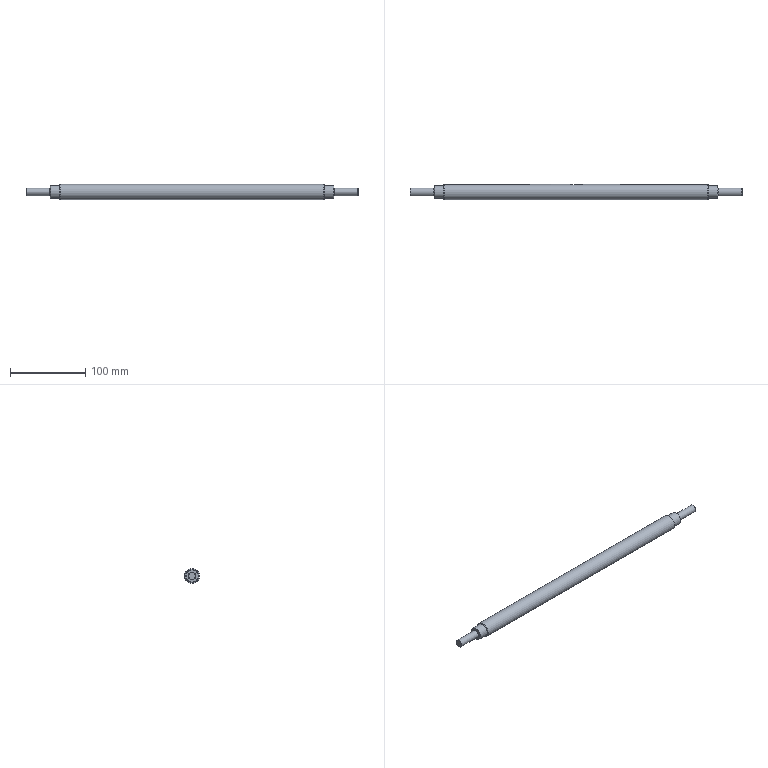Part | NX | features 5003_012_SFRJ20-350.0-F45.0-H13.0-G17-P10-T45.0-Z13.0-V17-Q10-KC166.0-A16(Default) 2 | 1 solid | 30 faces | box 440 x 20 x 20 mm | volume 120553 mm3 | plane 9 | cylinder 9 | cone 6 | torus 6 | commonest cylinder face diameters 0.4 x2 6 x2 10 x2 17 x2 20 x1
STEP:
#1=CARTESIAN_POINT('',(218.525,124.,-142.5));
#2=VERTEX_POINT('',#1);
#3=CARTESIAN_POINT('',(218.525,124.,-147.));
#4=DIRECTION('',(-1.,0.,0.));
#5=DIRECTION('',(0.,0.,1.));
#6=AXIS2_PLACEMENT_3D('',#3,#4,#5);
#7=CIRCLE('',#6,4.5);
#8=EDGE_CURVE('',#2,#2,#7,.F.);
#9=ORIENTED_EDGE('',*,*,#8,.T.);
#10=EDGE_LOOP('',(#9));
#11=FACE_BOUND('',#10,.T.);
#12=CARTESIAN_POINT('',(218.525,124.,-147.));
#13=DIRECTION('',(-1.,0.,0.));
#14=DIRECTION('',(0.,0.,1.));
#15=AXIS2_PLACEMENT_3D('',#12,#13,#14);
#16=PLANE('',#15);
#17=ADVANCED_FACE('',(#11),#16,.F.);
#18=CARTESIAN_POINT('',(186.725,124.,-142.));
#19=VERTEX_POINT('',#18);
#20=CARTESIAN_POINT('',(186.725,124.,-147.));
#21=DIRECTION('',(-1.,0.,0.));
#22=DIRECTION('',(0.,0.,1.));
#23=AXIS2_PLACEMENT_3D('',#20,#21,#22);
#24=CIRCLE('',#23,5.);
#25=EDGE_CURVE('',#19,#19,#24,.F.);
#26=ORIENTED_EDGE('',*,*,#25,.T.);
#27=EDGE_LOOP('',(#26));
#28=FACE_BOUND('',#27,.T.);
#29=CARTESIAN_POINT('',(218.025,124.,-142.));
#30=VERTEX_POINT('',#29);
#31=CARTESIAN_POINT('',(218.025,124.,-147.));
#32=DIRECTION('',(-1.,0.,0.));
#33=DIRECTION('',(0.,0.,1.));
#34=AXIS2_PLACEMENT_3D('',#31,#32,#33);
#35=CIRCLE('',#34,5.);
#36=EDGE_CURVE('',#30,#30,#35,.T.);
#37=ORIENTED_EDGE('',*,*,#36,.T.);
#38=EDGE_LOOP('',(#37));
#39=FACE_BOUND('',#38,.T.);
#40=CARTESIAN_POINT('',(218.525,124.,-147.));
#41=DIRECTION('',(1.,0.,0.));
#42=DIRECTION('',(0.,0.,-1.));
#43=AXIS2_PLACEMENT_3D('',#40,#41,#42);
#44=CYLINDRICAL_SURFACE('',#43,5.);
#45=ADVANCED_FACE('',(#28,#39),#44,.T.);
#46=CARTESIAN_POINT('',(186.525,124.,-141.8));
#47=VERTEX_POINT('',#46);
#48=CARTESIAN_POINT('',(186.525,124.,-147.));
#49=DIRECTION('',(-1.,0.,0.));
#50=DIRECTION('',(0.,0.,1.));
#51=AXIS2_PLACEMENT_3D('',#48,#49,#50);
#52=CIRCLE('',#51,5.2);
#53=EDGE_CURVE('',#47,#47,#52,.T.);
#54=ORIENTED_EDGE('',*,*,#53,.T.);
#55=EDGE_LOOP('',(#54));
#56=FACE_BOUND('',#55,.T.);
#57=CARTESIAN_POINT('',(186.525,124.,-139.));
#58=VERTEX_POINT('',#57);
#59=CARTESIAN_POINT('',(186.525,124.,-147.));
#60=DIRECTION('',(-1.,0.,0.));
#61=DIRECTION('',(0.,0.,1.));
#62=AXIS2_PLACEMENT_3D('',#59,#60,#61);
#63=CIRCLE('',#62,8.);
#64=EDGE_CURVE('',#58,#58,#63,.F.);
#65=ORIENTED_EDGE('',*,*,#64,.T.);
#66=EDGE_LOOP('',(#65));
#67=FACE_BOUND('',#66,.T.);
#68=CARTESIAN_POINT('',(186.525,124.,-142.));
#69=DIRECTION('',(-1.,0.,0.));
#70=DIRECTION('',(0.,0.,1.));
#71=AXIS2_PLACEMENT_3D('',#68,#69,#70);
#72=PLANE('',#71);
#73=ADVANCED_FACE('',(#56,#67),#72,.F.);
#74=CARTESIAN_POINT('',(173.725,124.,-138.5));
#75=VERTEX_POINT('',#74);
#76=CARTESIAN_POINT('',(173.725,124.,-147.));
#77=DIRECTION('',(-1.,0.,0.));
#78=DIRECTION('',(0.,0.,1.));
#79=AXIS2_PLACEMENT_3D('',#76,#77,#78);
#80=CIRCLE('',#79,8.5);
#81=EDGE_CURVE('',#75,#75,#80,.F.);
#82=ORIENTED_EDGE('',*,*,#81,.T.);
#83=EDGE_LOOP('',(#82));
#84=FACE_BOUND('',#83,.T.);
#85=CARTESIAN_POINT('',(186.025,124.,-138.5));
#86=VERTEX_POINT('',#85);
#87=CARTESIAN_POINT('',(186.025,124.,-147.));
#88=DIRECTION('',(-1.,0.,0.));
#89=DIRECTION('',(0.,0.,1.));
#90=AXIS2_PLACEMENT_3D('',#87,#88,#89);
#91=CIRCLE('',#90,8.5);
#92=EDGE_CURVE('',#86,#86,#91,.T.);
#93=ORIENTED_EDGE('',*,*,#92,.T.);
#94=EDGE_LOOP('',(#93));
#95=FACE_BOUND('',#94,.T.);
#96=CARTESIAN_POINT('',(218.525,124.,-147.));
#97=DIRECTION('',(1.,0.,0.));
#98=DIRECTION('',(0.,0.,-1.));
#99=AXIS2_PLACEMENT_3D('',#96,#97,#98);
#100=CYLINDRICAL_SURFACE('',#99,8.5);
#101=ADVANCED_FACE('',(#84,#95),#100,.T.);
#102=CARTESIAN_POINT('',(173.525,124.,-138.3));
#103=VERTEX_POINT('',#102);
#104=CARTESIAN_POINT('',(173.525,124.,-147.));
#105=DIRECTION('',(-1.,0.,0.));
#106=DIRECTION('',(0.,0.,1.));
#107=AXIS2_PLACEMENT_3D('',#104,#105,#106);
#108=CIRCLE('',#107,8.7);
#109=EDGE_CURVE('',#103,#103,#108,.T.);
#110=ORIENTED_EDGE('',*,*,#109,.T.);
#111=EDGE_LOOP('',(#110));
#112=FACE_BOUND('',#111,.T.);
#113=CARTESIAN_POINT('',(173.525,124.,-137.5));
#114=VERTEX_POINT('',#113);
#115=CARTESIAN_POINT('',(173.525,124.,-147.));
#116=DIRECTION('',(-1.,0.,0.));
#117=DIRECTION('',(0.,0.,1.));
#118=AXIS2_PLACEMENT_3D('',#115,#116,#117);
#119=CIRCLE('',#118,9.5);
#120=EDGE_CURVE('',#114,#114,#119,.F.);
#121=ORIENTED_EDGE('',*,*,#120,.T.);
#122=EDGE_LOOP('',(#121));
#123=FACE_BOUND('',#122,.T.);
#124=CARTESIAN_POINT('',(173.525,124.,-138.5));
#125=DIRECTION('',(-1.,0.,0.));
#126=DIRECTION('',(0.,0.,1.));
#127=AXIS2_PLACEMENT_3D('',#124,#125,#126);
#128=PLANE('',#127);
#129=ADVANCED_FACE('',(#112,#123),#128,.F.);
#130=CARTESIAN_POINT('',(4.525,133.539,-144.));
#131=VERTEX_POINT('',#130);
#132=CARTESIAN_POINT('',(-5.475,133.539,-144.));
#133=VERTEX_POINT('',#132);
#134=CARTESIAN_POINT('',(218.525,133.539,-144.));
#135=DIRECTION('',(1.,0.,0.));
#136=VECTOR('',#135,1000.);
#137=LINE('',#134,#136);
#138=EDGE_CURVE('',#131,#133,#137,.F.);
#139=ORIENTED_EDGE('',*,*,#138,.T.);
#140=CARTESIAN_POINT('',(-5.475,133.539,-150.));
#141=VERTEX_POINT('',#140);
#142=CARTESIAN_POINT('',(-5.475,133.539,-144.));
#143=CARTESIAN_POINT('',(-6.273,133.539,-144.));
#144=CARTESIAN_POINT('',(-7.819,133.775,-144.65));
#145=CARTESIAN_POINT('',(-8.803,134.112,-146.995));
#146=CARTESIAN_POINT('',(-7.82,133.775,-149.351));
#147=CARTESIAN_POINT('',(-6.273,133.539,-150.));
#148=CARTESIAN_POINT('',(-5.475,133.539,-150.));
#149=B_SPLINE_CURVE_WITH_KNOTS('',3,(#142,#143,#144,#145,#146,#147,#148),.UNSPECIFIED.,.F.,.F.,(4,1,1,1,4),(0.,0.002358,0.004715,0.007073,0.009431),.UNSPECIFIED.);
#150=EDGE_CURVE('',#133,#141,#149,.T.);
#151=ORIENTED_EDGE('',*,*,#150,.T.);
#152=CARTESIAN_POINT('',(4.525,133.539,-150.));
#153=VERTEX_POINT('',#152);
#154=CARTESIAN_POINT('',(218.525,133.539,-150.));
#155=DIRECTION('',(1.,0.,0.));
#156=VECTOR('',#155,1000.);
#157=LINE('',#154,#156);
#158=EDGE_CURVE('',#141,#153,#157,.T.);
#159=ORIENTED_EDGE('',*,*,#158,.T.);
#160=CARTESIAN_POINT('',(4.525,133.539,-150.));
#161=CARTESIAN_POINT('',(5.323,133.539,-150.));
#162=CARTESIAN_POINT('',(6.869,133.775,-149.35));
#163=CARTESIAN_POINT('',(7.853,134.112,-147.005));
#164=CARTESIAN_POINT('',(6.87,133.775,-144.649));
#165=CARTESIAN_POINT('',(5.323,133.539,-144.));
#166=CARTESIAN_POINT('',(4.525,133.539,-144.));
#167=B_SPLINE_CURVE_WITH_KNOTS('',3,(#160,#161,#162,#163,#164,#165,#166),.UNSPECIFIED.,.F.,.F.,(4,1,1,1,4),(0.,0.002358,0.004715,0.007073,0.009431),.UNSPECIFIED.);
#168=EDGE_CURVE('',#153,#131,#167,.T.);
#169=ORIENTED_EDGE('',*,*,#168,.T.);
#170=EDGE_LOOP('',(#139,#151,#159,#169));
#171=FACE_BOUND('',#170,.T.);
#172=CARTESIAN_POINT('',(-175.975,124.,-157.));
#173=VERTEX_POINT('',#172);
#174=CARTESIAN_POINT('',(-175.975,124.,-147.));
#175=DIRECTION('',(1.,0.,0.));
#176=DIRECTION('',(0.,0.,-1.));
#177=AXIS2_PLACEMENT_3D('',#174,#175,#176);
#178=CIRCLE('',#177,10.);
#179=EDGE_CURVE('',#173,#173,#178,.T.);
#180=ORIENTED_EDGE('',*,*,#179,.T.);
#181=EDGE_LOOP('',(#180));
#182=FACE_BOUND('',#181,.T.);
#183=CARTESIAN_POINT('',(173.025,124.,-137.));
#184=VERTEX_POINT('',#183);
#185=CARTESIAN_POINT('',(173.025,124.,-147.));
#186=DIRECTION('',(-1.,0.,0.));
#187=DIRECTION('',(0.,0.,1.));
#188=AXIS2_PLACEMENT_3D('',#185,#186,#187);
#189=CIRCLE('',#188,10.);
#190=EDGE_CURVE('',#184,#184,#189,.T.);
#191=ORIENTED_EDGE('',*,*,#190,.T.);
#192=EDGE_LOOP('',(#191));
#193=FACE_BOUND('',#192,.T.);
#194=CARTESIAN_POINT('',(218.525,124.,-147.));
#195=DIRECTION('',(1.,0.,0.));
#196=DIRECTION('',(0.,0.,-1.));
#197=AXIS2_PLACEMENT_3D('',#194,#195,#196);
#198=CYLINDRICAL_SURFACE('',#197,10.);
#199=ADVANCED_FACE('',(#171,#182,#193),#198,.T.);
#200=CARTESIAN_POINT('',(-176.475,124.,-155.7));
#201=VERTEX_POINT('',#200);
#202=CARTESIAN_POINT('',(-176.475,124.,-147.));
#203=DIRECTION('',(1.,0.,0.));
#204=DIRECTION('',(0.,0.,-1.));
#205=AXIS2_PLACEMENT_3D('',#202,#203,#204);
#206=CIRCLE('',#205,8.7);
#207=EDGE_CURVE('',#201,#201,#206,.T.);
#208=ORIENTED_EDGE('',*,*,#207,.T.);
#209=EDGE_LOOP('',(#208));
#210=FACE_BOUND('',#209,.T.);
#211=CARTESIAN_POINT('',(-176.475,124.,-156.5));
#212=VERTEX_POINT('',#211);
#213=CARTESIAN_POINT('',(-176.475,124.,-147.));
#214=DIRECTION('',(1.,0.,0.));
#215=DIRECTION('',(0.,0.,-1.));
#216=AXIS2_PLACEMENT_3D('',#213,#214,#215);
#217=CIRCLE('',#216,9.5);
#218=EDGE_CURVE('',#212,#212,#217,.F.);
#219=ORIENTED_EDGE('',*,*,#218,.T.);
#220=EDGE_LOOP('',(#219));
#221=FACE_BOUND('',#220,.T.);
#222=CARTESIAN_POINT('',(-176.475,124.,-137.));
#223=DIRECTION('',(1.,0.,0.));
#224=DIRECTION('',(0.,0.,-1.));
#225=AXIS2_PLACEMENT_3D('',#222,#223,#224);
#226=PLANE('',#225);
#227=ADVANCED_FACE('',(#210,#221),#226,.F.);
#228=CARTESIAN_POINT('',(-176.675,124.,-155.5));
#229=VERTEX_POINT('',#228);
#230=CARTESIAN_POINT('',(-176.675,124.,-147.));
#231=DIRECTION('',(1.,0.,0.));
#232=DIRECTION('',(0.,0.,-1.));
#233=AXIS2_PLACEMENT_3D('',#230,#231,#232);
#234=CIRCLE('',#233,8.5);
#235=EDGE_CURVE('',#229,#229,#234,.F.);
#236=ORIENTED_EDGE('',*,*,#235,.T.);
#237=EDGE_LOOP('',(#236));
#238=FACE_BOUND('',#237,.T.);
#239=CARTESIAN_POINT('',(-188.975,124.,-155.5));
#240=VERTEX_POINT('',#239);
#241=CARTESIAN_POINT('',(-188.975,124.,-147.));
#242=DIRECTION('',(1.,0.,0.));
#243=DIRECTION('',(0.,0.,-1.));
#244=AXIS2_PLACEMENT_3D('',#241,#242,#243);
#245=CIRCLE('',#244,8.5);
#246=EDGE_CURVE('',#240,#240,#245,.T.);
#247=ORIENTED_EDGE('',*,*,#246,.T.);
#248=EDGE_LOOP('',(#247));
#249=FACE_BOUND('',#248,.T.);
#250=CARTESIAN_POINT('',(218.525,124.,-147.));
#251=DIRECTION('',(1.,0.,0.));
#252=DIRECTION('',(0.,0.,-1.));
#253=AXIS2_PLACEMENT_3D('',#250,#251,#252);
#254=CYLINDRICAL_SURFACE('',#253,8.5);
#255=ADVANCED_FACE('',(#238,#249),#254,.T.);
#256=CARTESIAN_POINT('',(-189.475,124.,-152.2));
#257=VERTEX_POINT('',#256);
#258=CARTESIAN_POINT('',(-189.475,124.,-147.));
#259=DIRECTION('',(1.,0.,0.));
#260=DIRECTION('',(0.,0.,-1.));
#261=AXIS2_PLACEMENT_3D('',#258,#259,#260);
#262=CIRCLE('',#261,5.2);
#263=EDGE_CURVE('',#257,#257,#262,.T.);
#264=ORIENTED_EDGE('',*,*,#263,.T.);
#265=EDGE_LOOP('',(#264));
#266=FACE_BOUND('',#265,.T.);
#267=CARTESIAN_POINT('',(-189.475,124.,-155.));
#268=VERTEX_POINT('',#267);
#269=CARTESIAN_POINT('',(-189.475,124.,-147.));
#270=DIRECTION('',(1.,0.,0.));
#271=DIRECTION('',(0.,0.,-1.));
#272=AXIS2_PLACEMENT_3D('',#269,#270,#271);
#273=CIRCLE('',#272,8.);
#274=EDGE_CURVE('',#268,#268,#273,.F.);
#275=ORIENTED_EDGE('',*,*,#274,.T.);
#276=EDGE_LOOP('',(#275));
#277=FACE_BOUND('',#276,.T.);
#278=CARTESIAN_POINT('',(-189.475,124.,-138.5));
#279=DIRECTION('',(1.,0.,0.));
#280=DIRECTION('',(0.,0.,-1.));
#281=AXIS2_PLACEMENT_3D('',#278,#279,#280);
#282=PLANE('',#281);
#283=ADVANCED_FACE('',(#266,#277),#282,.F.);
#284=CARTESIAN_POINT('',(-189.675,124.,-152.));
#285=VERTEX_POINT('',#284);
#286=CARTESIAN_POINT('',(-189.675,124.,-147.));
#287=DIRECTION('',(1.,0.,0.));
#288=DIRECTION('',(0.,0.,-1.));
#289=AXIS2_PLACEMENT_3D('',#286,#287,#288);
#290=CIRCLE('',#289,5.);
#291=EDGE_CURVE('',#285,#285,#290,.F.);
#292=ORIENTED_EDGE('',*,*,#291,.T.);
#293=EDGE_LOOP('',(#292));
#294=FACE_BOUND('',#293,.T.);
#295=CARTESIAN_POINT('',(-220.975,124.,-152.));
#296=VERTEX_POINT('',#295);
#297=CARTESIAN_POINT('',(-220.975,124.,-147.));
#298=DIRECTION('',(1.,0.,0.));
#299=DIRECTION('',(0.,0.,-1.));
#300=AXIS2_PLACEMENT_3D('',#297,#298,#299);
#301=CIRCLE('',#300,5.);
#302=EDGE_CURVE('',#296,#296,#301,.T.);
#303=ORIENTED_EDGE('',*,*,#302,.T.);
#304=EDGE_LOOP('',(#303));
#305=FACE_BOUND('',#304,.T.);
#306=CARTESIAN_POINT('',(218.525,124.,-147.));
#307=DIRECTION('',(1.,0.,0.));
#308=DIRECTION('',(0.,0.,-1.));
#309=AXIS2_PLACEMENT_3D('',#306,#307,#308);
#310=CYLINDRICAL_SURFACE('',#309,5.);
#311=ADVANCED_FACE('',(#294,#305),#310,.T.);
#312=CARTESIAN_POINT('',(-221.475,124.,-151.5));
#313=VERTEX_POINT('',#312);
#314=CARTESIAN_POINT('',(-221.475,124.,-147.));
#315=DIRECTION('',(1.,0.,0.));
#316=DIRECTION('',(0.,0.,-1.));
#317=AXIS2_PLACEMENT_3D('',#314,#315,#316);
#318=CIRCLE('',#317,4.5);
#319=EDGE_CURVE('',#313,#313,#318,.F.);
#320=ORIENTED_EDGE('',*,*,#319,.T.);
#321=EDGE_LOOP('',(#320));
#322=FACE_BOUND('',#321,.T.);
#323=CARTESIAN_POINT('',(-221.475,124.,-142.));
#324=DIRECTION('',(1.,0.,0.));
#325=DIRECTION('',(0.,0.,-1.));
#326=AXIS2_PLACEMENT_3D('',#323,#324,#325);
#327=PLANE('',#326);
#328=ADVANCED_FACE('',(#322),#327,.F.);
#329=ORIENTED_EDGE('',*,*,#190,.F.);
#330=EDGE_LOOP('',(#329));
#331=FACE_BOUND('',#330,.T.);
#332=ORIENTED_EDGE('',*,*,#120,.F.);
#333=EDGE_LOOP('',(#332));
#334=FACE_BOUND('',#333,.T.);
#335=CARTESIAN_POINT('',(173.525,124.,-147.));
#336=DIRECTION('',(-1.,0.,0.));
#337=DIRECTION('',(0.,0.,1.));
#338=AXIS2_PLACEMENT_3D('',#335,#336,#337);
#339=CONICAL_SURFACE('',#338,9.5,0.7854);
#340=ADVANCED_FACE('',(#331,#334),#339,.T.);
#341=ORIENTED_EDGE('',*,*,#218,.F.);
#342=EDGE_LOOP('',(#341));
#343=FACE_BOUND('',#342,.T.);
#344=ORIENTED_EDGE('',*,*,#179,.F.);
#345=EDGE_LOOP('',(#344));
#346=FACE_BOUND('',#345,.T.);
#347=CARTESIAN_POINT('',(-175.975,124.,-147.));
#348=DIRECTION('',(1.,0.,0.));
#349=DIRECTION('',(0.,0.,-1.));
#350=AXIS2_PLACEMENT_3D('',#347,#348,#349);
#351=CONICAL_SURFACE('',#350,10.,0.7854);
#352=ADVANCED_FACE('',(#343,#346),#351,.T.);
#353=ORIENTED_EDGE('',*,*,#92,.F.);
#354=EDGE_LOOP('',(#353));
#355=FACE_BOUND('',#354,.T.);
#356=ORIENTED_EDGE('',*,*,#64,.F.);
#357=EDGE_LOOP('',(#356));
#358=FACE_BOUND('',#357,.T.);
#359=CARTESIAN_POINT('',(186.525,124.,-147.));
#360=DIRECTION('',(-1.,0.,0.));
#361=DIRECTION('',(0.,0.,1.));
#362=AXIS2_PLACEMENT_3D('',#359,#360,#361);
#363=CONICAL_SURFACE('',#362,8.,0.7854);
#364=ADVANCED_FACE('',(#355,#358),#363,.T.);
#365=ORIENTED_EDGE('',*,*,#274,.F.);
#366=EDGE_LOOP('',(#365));
#367=FACE_BOUND('',#366,.T.);
#368=ORIENTED_EDGE('',*,*,#246,.F.);
#369=EDGE_LOOP('',(#368));
#370=FACE_BOUND('',#369,.T.);
#371=CARTESIAN_POINT('',(-188.975,124.,-147.));
#372=DIRECTION('',(1.,0.,0.));
#373=DIRECTION('',(0.,0.,-1.));
#374=AXIS2_PLACEMENT_3D('',#371,#372,#373);
#375=CONICAL_SURFACE('',#374,8.5,0.7854);
#376=ADVANCED_FACE('',(#367,#370),#375,.T.);
#377=ORIENTED_EDGE('',*,*,#319,.F.);
#378=EDGE_LOOP('',(#377));
#379=FACE_BOUND('',#378,.T.);
#380=ORIENTED_EDGE('',*,*,#302,.F.);
#381=EDGE_LOOP('',(#380));
#382=FACE_BOUND('',#381,.T.);
#383=CARTESIAN_POINT('',(-220.975,124.,-147.));
#384=DIRECTION('',(1.,0.,0.));
#385=DIRECTION('',(0.,0.,-1.));
#386=AXIS2_PLACEMENT_3D('',#383,#384,#385);
#387=CONICAL_SURFACE('',#386,5.,0.7854);
#388=ADVANCED_FACE('',(#379,#382),#387,.T.);
#389=ORIENTED_EDGE('',*,*,#36,.F.);
#390=EDGE_LOOP('',(#389));
#391=FACE_BOUND('',#390,.T.);
#392=ORIENTED_EDGE('',*,*,#8,.F.);
#393=EDGE_LOOP('',(#392));
#394=FACE_BOUND('',#393,.T.);
#395=CARTESIAN_POINT('',(218.525,124.,-147.));
#396=DIRECTION('',(-1.,0.,0.));
#397=DIRECTION('',(0.,0.,1.));
#398=AXIS2_PLACEMENT_3D('',#395,#396,#397);
#399=CONICAL_SURFACE('',#398,4.5,0.7854);
#400=ADVANCED_FACE('',(#391,#394),#399,.T.);
#401=ORIENTED_EDGE('',*,*,#291,.F.);
#402=EDGE_LOOP('',(#401));
#403=FACE_BOUND('',#402,.T.);
#404=ORIENTED_EDGE('',*,*,#263,.F.);
#405=EDGE_LOOP('',(#404));
#406=FACE_BOUND('',#405,.T.);
#407=CARTESIAN_POINT('',(-189.675,124.,-147.));
#408=DIRECTION('',(1.,0.,0.));
#409=DIRECTION('',(0.,0.,-1.));
#410=AXIS2_PLACEMENT_3D('',#407,#408,#409);
#411=TOROIDAL_SURFACE('',#410,5.2,0.2);
#412=ADVANCED_FACE('',(#403,#406),#411,.F.);
#413=ORIENTED_EDGE('',*,*,#235,.F.);
#414=EDGE_LOOP('',(#413));
#415=FACE_BOUND('',#414,.T.);
#416=ORIENTED_EDGE('',*,*,#207,.F.);
#417=EDGE_LOOP('',(#416));
#418=FACE_BOUND('',#417,.T.);
#419=CARTESIAN_POINT('',(-176.675,124.,-147.));
#420=DIRECTION('',(1.,0.,0.));
#421=DIRECTION('',(0.,0.,-1.));
#422=AXIS2_PLACEMENT_3D('',#419,#420,#421);
#423=TOROIDAL_SURFACE('',#422,8.7,0.2);
#424=ADVANCED_FACE('',(#415,#418),#423,.F.);
#425=ORIENTED_EDGE('',*,*,#109,.F.);
#426=EDGE_LOOP('',(#425));
#427=FACE_BOUND('',#426,.T.);
#428=ORIENTED_EDGE('',*,*,#81,.F.);
#429=EDGE_LOOP('',(#428));
#430=FACE_BOUND('',#429,.T.);
#431=CARTESIAN_POINT('',(173.725,124.,-147.));
#432=DIRECTION('',(-1.,0.,0.));
#433=DIRECTION('',(0.,0.,1.));
#434=AXIS2_PLACEMENT_3D('',#431,#432,#433);
#435=TOROIDAL_SURFACE('',#434,8.7,0.2);
#436=ADVANCED_FACE('',(#427,#430),#435,.F.);
#437=ORIENTED_EDGE('',*,*,#53,.F.);
#438=EDGE_LOOP('',(#437));
#439=FACE_BOUND('',#438,.T.);
#440=ORIENTED_EDGE('',*,*,#25,.F.);
#441=EDGE_LOOP('',(#440));
#442=FACE_BOUND('',#441,.T.);
#443=CARTESIAN_POINT('',(186.725,124.,-147.));
#444=DIRECTION('',(-1.,0.,0.));
#445=DIRECTION('',(0.,0.,1.));
#446=AXIS2_PLACEMENT_3D('',#443,#444,#445);
#447=TOROIDAL_SURFACE('',#446,5.2,0.2);
#448=ADVANCED_FACE('',(#439,#442),#447,.F.);
#449=CARTESIAN_POINT('',(-5.475,130.7,-144.));
#450=VERTEX_POINT('',#449);
#451=CARTESIAN_POINT('',(-5.475,130.5,-144.));
#452=DIRECTION('',(0.,1.,0.));
#453=VECTOR('',#452,1000.);
#454=LINE('',#451,#453);
#455=EDGE_CURVE('',#133,#450,#454,.F.);
#456=ORIENTED_EDGE('',*,*,#455,.T.);
#457=CARTESIAN_POINT('',(-5.475,130.7,-150.));
#458=VERTEX_POINT('',#457);
#459=CARTESIAN_POINT('',(-5.475,130.7,-147.));
#460=DIRECTION('',(0.,1.,0.));
#461=DIRECTION('',(-1.,0.,0.));
#462=AXIS2_PLACEMENT_3D('',#459,#460,#461);
#463=CIRCLE('',#462,3.);
#464=EDGE_CURVE('',#458,#450,#463,.T.);
#465=ORIENTED_EDGE('',*,*,#464,.F.);
#466=CARTESIAN_POINT('',(-5.475,130.5,-150.));
#467=DIRECTION('',(0.,1.,0.));
#468=VECTOR('',#467,1000.);
#469=LINE('',#466,#468);
#470=EDGE_CURVE('',#458,#141,#469,.T.);
#471=ORIENTED_EDGE('',*,*,#470,.T.);
#472=ORIENTED_EDGE('',*,*,#150,.F.);
#473=EDGE_LOOP('',(#456,#465,#471,#472));
#474=FACE_BOUND('',#473,.T.);
#475=CARTESIAN_POINT('',(-5.475,134.,-147.));
#476=DIRECTION('',(0.,1.,0.));
#477=DIRECTION('',(-1.,0.,0.));
#478=AXIS2_PLACEMENT_3D('',#475,#476,#477);
#479=CYLINDRICAL_SURFACE('',#478,3.);
#480=ADVANCED_FACE('',(#474),#479,.F.);
#481=CARTESIAN_POINT('',(4.525,130.7,-150.));
#482=VERTEX_POINT('',#481);
#483=CARTESIAN_POINT('',(4.525,130.5,-150.));
#484=DIRECTION('',(0.,1.,0.));
#485=VECTOR('',#484,1000.);
#486=LINE('',#483,#485);
#487=EDGE_CURVE('',#153,#482,#486,.F.);
#488=ORIENTED_EDGE('',*,*,#487,.T.);
#489=CARTESIAN_POINT('',(4.525,130.7,-144.));
#490=VERTEX_POINT('',#489);
#491=CARTESIAN_POINT('',(4.525,130.7,-147.));
#492=DIRECTION('',(0.,1.,0.));
#493=DIRECTION('',(-1.,0.,0.));
#494=AXIS2_PLACEMENT_3D('',#491,#492,#493);
#495=CIRCLE('',#494,3.);
#496=EDGE_CURVE('',#490,#482,#495,.T.);
#497=ORIENTED_EDGE('',*,*,#496,.F.);
#498=CARTESIAN_POINT('',(4.525,130.5,-144.));
#499=DIRECTION('',(0.,1.,0.));
#500=VECTOR('',#499,1000.);
#501=LINE('',#498,#500);
#502=EDGE_CURVE('',#490,#131,#501,.T.);
#503=ORIENTED_EDGE('',*,*,#502,.T.);
#504=ORIENTED_EDGE('',*,*,#168,.F.);
#505=EDGE_LOOP('',(#488,#497,#503,#504));
#506=FACE_BOUND('',#505,.T.);
#507=CARTESIAN_POINT('',(4.525,130.5,-147.));
#508=DIRECTION('',(0.,1.,0.));
#509=DIRECTION('',(-1.,0.,0.));
#510=AXIS2_PLACEMENT_3D('',#507,#508,#509);
#511=CYLINDRICAL_SURFACE('',#510,3.);
#512=ADVANCED_FACE('',(#506),#511,.F.);
#513=ORIENTED_EDGE('',*,*,#502,.F.);
#514=CARTESIAN_POINT('',(4.525,130.7,-144.));
#515=DIRECTION('',(1.,0.,0.));
#516=VECTOR('',#515,1000.);
#517=LINE('',#514,#516);
#518=EDGE_CURVE('',#450,#490,#517,.T.);
#519=ORIENTED_EDGE('',*,*,#518,.F.);
#520=ORIENTED_EDGE('',*,*,#455,.F.);
#521=ORIENTED_EDGE('',*,*,#138,.F.);
#522=EDGE_LOOP('',(#513,#519,#520,#521));
#523=FACE_BOUND('',#522,.T.);
#524=CARTESIAN_POINT('',(7.525,130.5,-144.));
#525=DIRECTION('',(0.,0.,1.));
#526=DIRECTION('',(1.,0.,0.));
#527=AXIS2_PLACEMENT_3D('',#524,#525,#526);
#528=PLANE('',#527);
#529=ADVANCED_FACE('',(#523),#528,.F.);
#530=ORIENTED_EDGE('',*,*,#470,.F.);
#531=CARTESIAN_POINT('',(-5.475,130.7,-150.));
#532=DIRECTION('',(-1.,0.,0.));
#533=VECTOR('',#532,1000.);
#534=LINE('',#531,#533);
#535=EDGE_CURVE('',#482,#458,#534,.T.);
#536=ORIENTED_EDGE('',*,*,#535,.F.);
#537=ORIENTED_EDGE('',*,*,#487,.F.);
#538=ORIENTED_EDGE('',*,*,#158,.F.);
#539=EDGE_LOOP('',(#530,#536,#537,#538));
#540=FACE_BOUND('',#539,.T.);
#541=CARTESIAN_POINT('',(7.525,130.5,-150.));
#542=DIRECTION('',(0.,0.,-1.));
#543=DIRECTION('',(-1.,0.,0.));
#544=AXIS2_PLACEMENT_3D('',#541,#542,#543);
#545=PLANE('',#544);
#546=ADVANCED_FACE('',(#540),#545,.F.);
#547=CARTESIAN_POINT('',(4.525,130.5,-149.8));
#548=VERTEX_POINT('',#547);
#549=CARTESIAN_POINT('',(4.525,130.5,-144.2));
#550=VERTEX_POINT('',#549);
#551=CARTESIAN_POINT('',(4.525,130.5,-147.));
#552=DIRECTION('',(0.,1.,0.));
#553=DIRECTION('',(-1.,0.,0.));
#554=AXIS2_PLACEMENT_3D('',#551,#552,#553);
#555=CIRCLE('',#554,2.8);
#556=EDGE_CURVE('',#548,#550,#555,.F.);
#557=ORIENTED_EDGE('',*,*,#556,.F.);
#558=CARTESIAN_POINT('',(-5.475,130.5,-149.8));
#559=VERTEX_POINT('',#558);
#560=CARTESIAN_POINT('',(4.525,130.5,-149.8));
#561=DIRECTION('',(-1.,0.,0.));
#562=VECTOR('',#561,1000.);
#563=LINE('',#560,#562);
#564=EDGE_CURVE('',#559,#548,#563,.F.);
#565=ORIENTED_EDGE('',*,*,#564,.F.);
#566=CARTESIAN_POINT('',(-5.475,130.5,-144.2));
#567=VERTEX_POINT('',#566);
#568=CARTESIAN_POINT('',(-5.475,130.5,-147.));
#569=DIRECTION('',(0.,1.,0.));
#570=DIRECTION('',(-1.,0.,0.));
#571=AXIS2_PLACEMENT_3D('',#568,#569,#570);
#572=CIRCLE('',#571,2.8);
#573=EDGE_CURVE('',#567,#559,#572,.F.);
#574=ORIENTED_EDGE('',*,*,#573,.F.);
#575=CARTESIAN_POINT('',(-5.475,130.5,-144.2));
#576=DIRECTION('',(1.,0.,0.));
#577=VECTOR('',#576,1000.);
#578=LINE('',#575,#577);
#579=EDGE_CURVE('',#550,#567,#578,.F.);
#580=ORIENTED_EDGE('',*,*,#579,.F.);
#581=EDGE_LOOP('',(#557,#565,#574,#580));
#582=FACE_BOUND('',#581,.T.);
#583=CARTESIAN_POINT('',(218.525,130.5,-147.));
#584=DIRECTION('',(0.,1.,0.));
#585=DIRECTION('',(-1.,0.,0.));
#586=AXIS2_PLACEMENT_3D('',#583,#584,#585);
#587=PLANE('',#586);
#588=ADVANCED_FACE('',(#582),#587,.T.);
#589=CARTESIAN_POINT('',(4.525,130.7,-149.8));
#590=DIRECTION('',(1.,0.,0.));
#591=DIRECTION('',(0.,1.,0.));
#592=AXIS2_PLACEMENT_3D('',#589,#590,#591);
#593=CIRCLE('',#592,0.2);
#594=EDGE_CURVE('',#548,#482,#593,.T.);
#595=ORIENTED_EDGE('',*,*,#594,.T.);
#596=ORIENTED_EDGE('',*,*,#535,.T.);
#597=CARTESIAN_POINT('',(-5.475,130.7,-149.8));
#598=DIRECTION('',(-1.,0.,0.));
#599=DIRECTION('',(0.,-1.,0.));
#600=AXIS2_PLACEMENT_3D('',#597,#598,#599);
#601=CIRCLE('',#600,0.2);
#602=EDGE_CURVE('',#458,#559,#601,.T.);
#603=ORIENTED_EDGE('',*,*,#602,.T.);
#604=ORIENTED_EDGE('',*,*,#564,.T.);
#605=EDGE_LOOP('',(#595,#596,#603,#604));
#606=FACE_BOUND('',#605,.T.);
#607=CARTESIAN_POINT('',(7.525,130.7,-149.8));
#608=DIRECTION('',(1.,0.,0.));
#609=DIRECTION('',(0.,0.,-1.));
#610=AXIS2_PLACEMENT_3D('',#607,#608,#609);
#611=CYLINDRICAL_SURFACE('',#610,0.2);
#612=ADVANCED_FACE('',(#606),#611,.F.);
#613=ORIENTED_EDGE('',*,*,#602,.F.);
#614=ORIENTED_EDGE('',*,*,#464,.T.);
#615=CARTESIAN_POINT('',(-5.475,130.7,-144.2));
#616=DIRECTION('',(1.,0.,0.));
#617=DIRECTION('',(0.,1.,0.));
#618=AXIS2_PLACEMENT_3D('',#615,#616,#617);
#619=CIRCLE('',#618,0.2);
#620=EDGE_CURVE('',#450,#567,#619,.T.);
#621=ORIENTED_EDGE('',*,*,#620,.T.);
#622=ORIENTED_EDGE('',*,*,#573,.T.);
#623=EDGE_LOOP('',(#613,#614,#621,#622));
#624=FACE_BOUND('',#623,.T.);
#625=CARTESIAN_POINT('',(-5.475,130.7,-147.));
#626=DIRECTION('',(0.,1.,0.));
#627=DIRECTION('',(-1.,0.,0.));
#628=AXIS2_PLACEMENT_3D('',#625,#626,#627);
#629=TOROIDAL_SURFACE('',#628,2.8,0.2);
#630=ADVANCED_FACE('',(#624),#629,.F.);
#631=ORIENTED_EDGE('',*,*,#594,.F.);
#632=ORIENTED_EDGE('',*,*,#556,.T.);
#633=CARTESIAN_POINT('',(4.525,130.7,-144.2));
#634=DIRECTION('',(-1.,0.,0.));
#635=DIRECTION('',(0.,-1.,0.));
#636=AXIS2_PLACEMENT_3D('',#633,#634,#635);
#637=CIRCLE('',#636,0.2);
#638=EDGE_CURVE('',#550,#490,#637,.T.);
#639=ORIENTED_EDGE('',*,*,#638,.T.);
#640=ORIENTED_EDGE('',*,*,#496,.T.);
#641=EDGE_LOOP('',(#631,#632,#639,#640));
#642=FACE_BOUND('',#641,.T.);
#643=CARTESIAN_POINT('',(4.525,130.7,-147.));
#644=DIRECTION('',(0.,1.,0.));
#645=DIRECTION('',(-1.,0.,0.));
#646=AXIS2_PLACEMENT_3D('',#643,#644,#645);
#647=TOROIDAL_SURFACE('',#646,2.8,0.2);
#648=ADVANCED_FACE('',(#642),#647,.F.);
#649=ORIENTED_EDGE('',*,*,#620,.F.);
#650=ORIENTED_EDGE('',*,*,#518,.T.);
#651=ORIENTED_EDGE('',*,*,#638,.F.);
#652=ORIENTED_EDGE('',*,*,#579,.T.);
#653=EDGE_LOOP('',(#649,#650,#651,#652));
#654=FACE_BOUND('',#653,.T.);
#655=CARTESIAN_POINT('',(7.525,130.7,-144.2));
#656=DIRECTION('',(-1.,0.,0.));
#657=DIRECTION('',(0.,0.,1.));
#658=AXIS2_PLACEMENT_3D('',#655,#656,#657);
#659=CYLINDRICAL_SURFACE('',#658,0.2);
#660=ADVANCED_FACE('',(#654),#659,.F.);
#661=CLOSED_SHELL('',(#17,#45,#73,#101,#129,#199,#227,#255,#283,#311,#328,#340,#352,#364,#376,#388,#400,#412,#424,#436,#448,#480,#512,#529,#546,#588,#612,#630,#648,#660));
#662=MANIFOLD_SOLID_BREP('',#661);
#663=(LENGTH_UNIT()NAMED_UNIT(*)SI_UNIT(.MILLI.,.METRE.));
#664=UNCERTAINTY_MEASURE_WITH_UNIT(LENGTH_MEASURE(0.0508),#663,'','');
#665=(NAMED_UNIT(*)PLANE_ANGLE_UNIT()SI_UNIT($,.RADIAN.));
#666=(NAMED_UNIT(*)SI_UNIT($,.STERADIAN.)SOLID_ANGLE_UNIT());
#667=(GEOMETRIC_REPRESENTATION_CONTEXT(3)GLOBAL_UNCERTAINTY_ASSIGNED_CONTEXT((#664))GLOBAL_UNIT_ASSIGNED_CONTEXT((#663,#665,#666))REPRESENTATION_CONTEXT('',''));
#668=ADVANCED_BREP_SHAPE_REPRESENTATION('',(#662),#667);